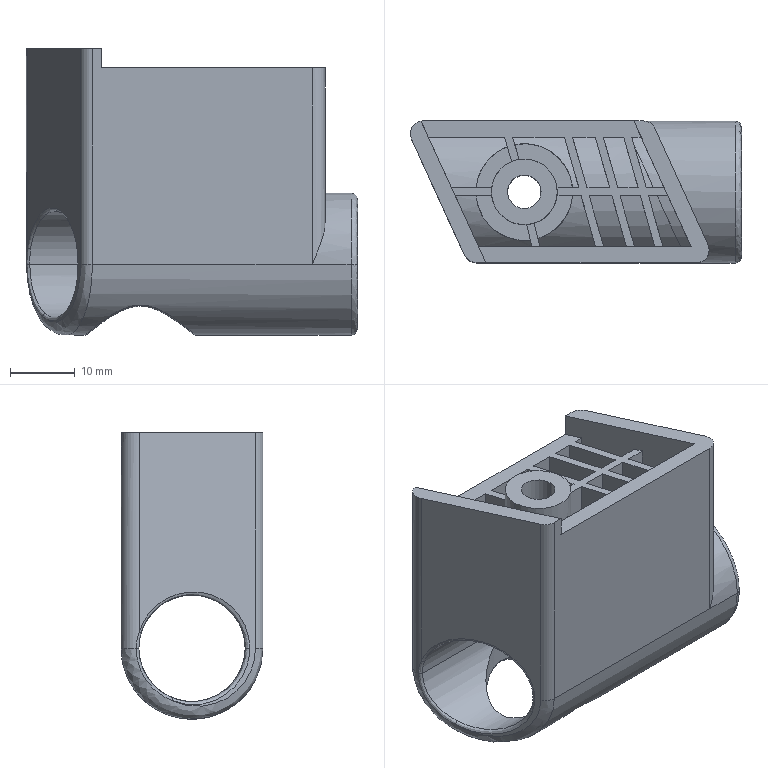Part | SolidWorks | features BaseBody 1 | 1 solid | 96 faces | box 51.079 x 21.892 x 44.191 mm | volume 16230 mm3 | plane 52 | cylinder 32 | spline 12 | commonest cylinder face diameters 21.394 x10 3.98 x4 14.926 x4 21.892 x4 5.174 x2 10.15 x2